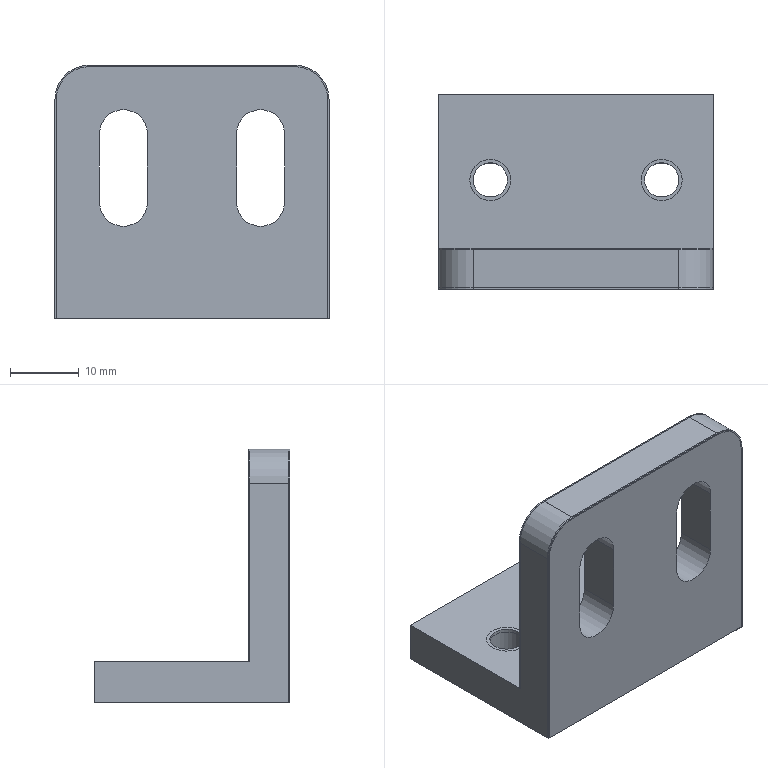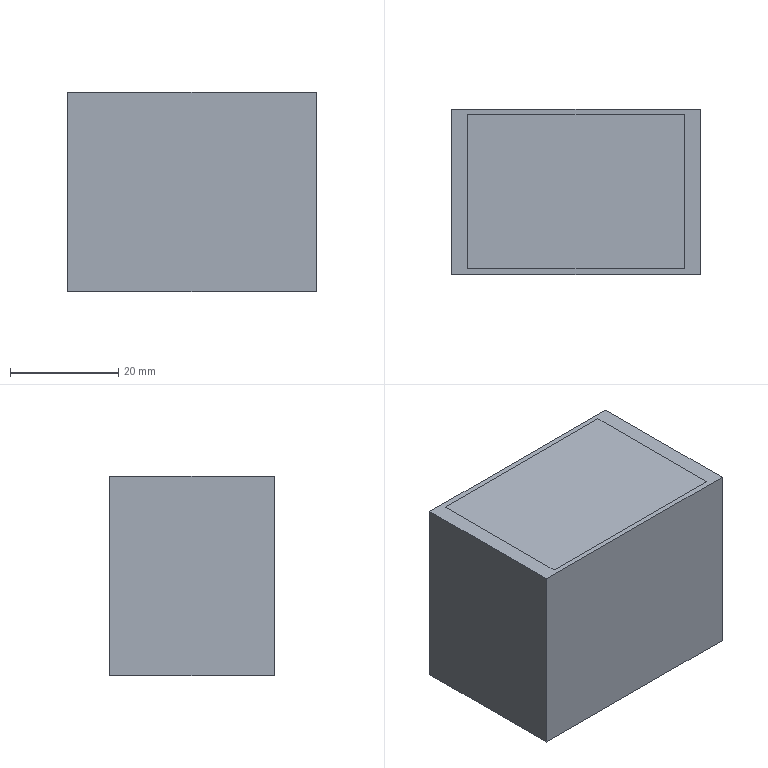CAM job | NX | 3+2 milling, drilling | part box 40 x 28.5 x 37 mm | stock box 46 x 30.5 x 37 mm
Tools:
number,name,description,diameter,corner_radius,flute_length,length,flutes
1,D16CU,Milling Tool-5 Parameters,16.0,0.0,50.0,75.0,2
2,D16.,Milling Tool-5 Parameters,16.0,0.0,50.0,75.0,2
3,D8点钻,Chamfer Mill,8.0,0.0,50.0,75.0,2
19,4倒角,Drilling Tool,4.0,0.0,35.0,50.0,2
6,Z5.1,Drilling Tool,5.1,0.0,35.0,50.0,2
7,M6,Drilling Tool,6.0,0.0,35.0,50.0,4
17,D3球刀,Milling Tool-Ball Mill,3.0,1.5,50.0,75.0,2
18,D63.,Milling Tool-5 Parameters,63.0,0.0,50.0,75.0,2
20,D63.J,Milling Tool-5 Parameters,63.0,0.0,50.0,75.0,2
5,D6.,Milling Tool-5 Parameters,6.0,0.0,50.0,75.0,2
20,SPHERICAL_MILL,Spherical Mill,6.0,3.0,5.437,20.0,2
6,D6J,Milling Tool-5 Parameters,6.0,0.0,50.0,75.0,2
Operations:
program,operation,operation_type,tool,method,geometry_group,spindle_rpm,surface_speed,feed_per_tooth,feed_cut,feed_plunge,cut_length_mm,path_length_mm,cut_time_min,machine_time_min
G54,FLOOR_FACING,VolumeBased25DMillingOperation,D16CU,METHOD,WORKPIECE,1500.0,471.0,0.1333,400.0,100.0,72.0,125.8,0.18,0.1854
G54,PLANAR_MILL_COPY_1_COPY_COPY,PlanarMilling,D16CU,METHOD,WORKPIECE,1300.0,65.0,0.5769,1500.0,100.0,420.0,1396.803,0.28,0.3777
G54,PLANAR_MILL_COPY_1_COPY_COPY_COPY,PlanarMilling,D16CU,METHOD,WORKPIECE,1300.0,65.0,0.5769,1500.0,100.0,630.5,2311.708,0.4203,0.5885
G54,PLANAR_MILL_COPY_1_COPY_COPY_COPY_1,PlanarMilling,D16CU,METHOD,WORKPIECE,1300.0,65.0,0.5769,1500.0,100.0,420.0,1396.803,0.28,0.3777
G54,PLANAR_MILL_COPY_1_COPY_COPY_COPY_COPY,PlanarMilling,D16CU,METHOD,WORKPIECE,1300.0,65.0,0.5769,1500.0,100.0,630.5,2311.708,0.4203,0.5885
G54,PLANAR_MILL_COPY_1_COPY_COPY_COPY_2,PlanarMilling,D16CU,METHOD,WORKPIECE,1300.0,65.0,0.5769,1500.0,100.0,60.0,194.4,0.04,0.0534
G54,PLANAR_MILL_COPY_1_COPY_COPY_COPY_1_COPY,PlanarMilling,D16CU,METHOD,WORKPIECE,1300.0,65.0,0.5769,1500.0,100.0,60.0,194.4,0.04,0.0534
G54,PLANAR_MILL_COPY_1_COPY_COPY_COPY_COPY_1,PlanarMilling,D16CU,METHOD,WORKPIECE,700.0,35.0,0.1429,200.0,100.0,48.5,182.9,0.2425,0.2559
G54,PLANAR_MILL_COPY_1_COPY_COPY_COPY_COPY_COPY,PlanarMilling,D16CU,METHOD,WORKPIECE,700.0,35.0,0.1429,200.0,100.0,48.5,182.9,0.2425,0.2559
G54,PLANAR_MILL,PlanarMilling,D16.,METHOD,WORKPIECE,1200.0,60.0,0.1667,400.0,100.0,391.07,525.47,0.9777,0.9911
G54,PLANAR_MILL_COPY,PlanarMilling,D16.,METHOD,WORKPIECE,800.0,40.0,0.125,200.0,100.0,390.692,525.092,1.954,1.967
G54,PLANAR_MILL_COPY_1_COPY,PlanarMilling,D16CU,METHOD,WORKPIECE,1500.0,75.0,0.5,1500.0,100.0,5460.0,17083.847,3.64,4.802
G54,FLOOR_FACING_COPY,VolumeBased25DMillingOperation,D16.,METHOD,WORKPIECE,2500.0,125.0,0.14,700.0,100.0,206.9,322.9,0.2956,0.3072
G54,FLOOR_FACING_COPY_1,VolumeBased25DMillingOperation,D16.,METHOD,WORKPIECE,2500.0,125.0,0.14,700.0,100.0,72.0,126.0,0.1029,0.1083
G54,PLANAR_MILL_COPY_1,PlanarMilling,D16.,METHOD,WORKPIECE,1200.0,60.0,0.1667,400.0,100.0,120.0,423.6,0.3,0.3304
G54,PLANAR_MILL_COPY_1_COPY_1,PlanarMilling,D16.,METHOD,WORKPIECE_3,1000.0,50.0,0.1,200.0,100.0,56.732,178.632,0.2837,0.2959
G54,PLANAR_MILL_COPY_COPY_1_1,PlanarMilling,4倒角,METHOD,WORKPIECE,4500.0,113.0,0.0889,800.0,100.0,91.063,216.063,0.1138,0.1263
G54,PLANAR_MILL_COPY_COPY_1_1_COPY,PlanarMilling,4倒角,METHOD,WORKPIECE,4500.0,113.0,0.0889,800.0,100.0,94.0,229.347,0.1175,0.131
G54,CURVE_DRIVE,SurfaceContour,D3球刀,METHOD,WORKPIECE,6000.0,56.0,0.0833,1000.0,100.0,513.234,570.422,0.5132,0.519
G54,CURVE_DRIVE_COPY,SurfaceContour,D3球刀,METHOD,WORKPIECE,6000.0,56.0,0.0833,1000.0,100.0,513.234,570.422,0.5132,0.519
G54,CURVE_DRIVE_COPY_1,SurfaceContour,D3球刀,METHOD,WORKPIECE_3,6000.0,56.0,0.0417,500.0,100.0,67.339,129.612,0.1347,0.1409
G54,CURVE_DRIVE_COPY_1_COPY,SurfaceContour,D3球刀,METHOD,WORKPIECE_3,6000.0,56.0,0.0417,500.0,100.0,67.389,129.634,0.1348,0.141
G55,FLOOR_FACING_COPY_2,VolumeBased25DMillingOperation,D63.,METHOD,WORKPIECE_4,1500.0,296.0,0.4,1200.0,100.0,1032.0,2626.6,0.86,1.02
G55,FLOOR_FACING_COPY_2_COPY,VolumeBased25DMillingOperation,D63.J,METHOD,WORKPIECE_4,1500.0,471.0,0.1333,400.0,100.0,129.0,223.0,0.3225,0.3319
G55,PLANAR_MILL_COPY_COPY_1_1_COPY_COPY,PlanarMilling,4倒角,METHOD,WORKPIECE_4,4500.0,113.0,0.0889,800.0,100.0,149.19,252.19,0.1865,0.1968
G55,DRILLING_COPY,Operation,D8点钻,METHOD,WORKPIECE_4,1500.0,37.0,0.0267,80.0,0.0,12.4,152.979,0.155,0.1691
G55,PECK_DRILLING_1,Operation,Z5.1,METHOD,WORKPIECE_4,1200.0,19.0,0.0333,80.0,0.0,36.0,160.179,0.45,0.4624
G55,PECK_DRILLING_COPY_1,Operation,M6,METHOD,WORKPIECE_4,200.0,3.0,0.0013,1.0,0.0,22.0,132.179,22.0,22.011
G56,PLANAR_MILL_1,PlanarMilling,D6.,METHOD,WORKPIECE_5,2500.0,47.0,0.24,1200.0,100.0,1165.549,1482.254,0.9713,1.003
G56,PLANAR_MILL_1_COPY,PlanarMilling,D6J,METHOD,WORKPIECE_5,2000.0,37.0,0.0375,150.0,100.0,102.508,432.509,0.6834,0.7164
G56,PLANAR_MILL_COPY_COPY_1_1_COPY_COPY_COPY,PlanarMilling,4倒角,METHOD,WORKPIECE_5,4500.0,113.0,0.0889,800.0,100.0,73.133,391.521,0.0914,0.1233
G56,CURVE_DRIVE_COPY_2,SurfaceContour,SPHERICAL_MILL,METHOD,WORKPIECE_5,3500.0,65.0,0.0086,60.0,100.0,17.52,148.52,0.292,0.3051
G56,CURVE_DRIVE_COPY_COPY,SurfaceContour,SPHERICAL_MILL,METHOD,WORKPIECE_5,3500.0,65.0,0.0086,60.0,100.0,17.52,148.52,0.292,0.3051
G56,CURVE_DRIVE_COPY_2_COPY,SurfaceContour,SPHERICAL_MILL,METHOD,WORKPIECE_5,3500.0,65.0,0.0086,60.0,100.0,17.609,148.609,0.2935,0.3066
G56,CURVE_DRIVE_COPY_COPY_COPY,SurfaceContour,SPHERICAL_MILL,METHOD,WORKPIECE_5,3500.0,65.0,0.0086,60.0,100.0,17.609,148.609,0.2935,0.3066